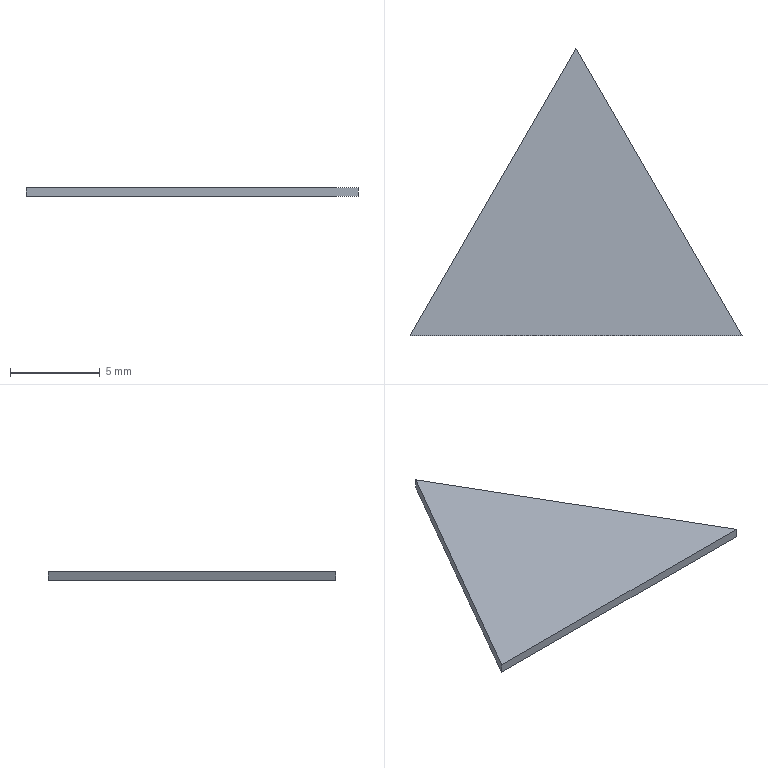Part | STEP file | [Hold-down mark] | 1 solid | 5 faces | box 18.475 x 16 x 0.5 mm | volume 73.901 mm3 | plane 5
STEP:
#1=CARTESIAN_POINT('',(0.,0.,0.5));
#2=VERTEX_POINT('',#1);
#3=CARTESIAN_POINT('',(9.238,16.,0.5));
#4=VERTEX_POINT('',#3);
#5=CARTESIAN_POINT('',(0.,0.,0.5));
#6=DIRECTION('',(0.5,0.866,0.));
#7=VECTOR('',#6,1000.);
#8=LINE('',#5,#7);
#9=EDGE_CURVE('',#2,#4,#8,.T.);
#10=ORIENTED_EDGE('',*,*,#9,.T.);
#11=CARTESIAN_POINT('',(9.238,16.,0.));
#12=VERTEX_POINT('',#11);
#13=CARTESIAN_POINT('',(9.238,16.,0.));
#14=DIRECTION('',(0.,0.,1.));
#15=VECTOR('',#14,1000.);
#16=LINE('',#13,#15);
#17=EDGE_CURVE('',#12,#4,#16,.T.);
#18=ORIENTED_EDGE('',*,*,#17,.F.);
#19=CARTESIAN_POINT('',(0.,0.,0.));
#20=VERTEX_POINT('',#19);
#21=CARTESIAN_POINT('',(0.,0.,0.));
#22=DIRECTION('',(0.5,0.866,0.));
#23=VECTOR('',#22,1000.);
#24=LINE('',#21,#23);
#25=EDGE_CURVE('',#20,#12,#24,.T.);
#26=ORIENTED_EDGE('',*,*,#25,.F.);
#27=CARTESIAN_POINT('',(0.,0.,0.));
#28=DIRECTION('',(0.,0.,1.));
#29=VECTOR('',#28,1000.);
#30=LINE('',#27,#29);
#31=EDGE_CURVE('',#20,#2,#30,.T.);
#32=ORIENTED_EDGE('',*,*,#31,.T.);
#33=EDGE_LOOP('',(#10,#18,#26,#32));
#34=FACE_OUTER_BOUND('',#33,.T.);
#35=CARTESIAN_POINT('',(0.,0.,0.));
#36=DIRECTION('',(0.866,-0.5,0.));
#37=DIRECTION('',(-0.5,-0.866,0.));
#38=AXIS2_PLACEMENT_3D('',#35,#36,#37);
#39=PLANE('',#38);
#40=ADVANCED_FACE('',(#34),#39,.F.);
#41=CARTESIAN_POINT('',(18.475,0.,0.5));
#42=VERTEX_POINT('',#41);
#43=CARTESIAN_POINT('',(9.238,16.,0.5));
#44=DIRECTION('',(0.5,-0.866,0.));
#45=VECTOR('',#44,1000.);
#46=LINE('',#43,#45);
#47=EDGE_CURVE('',#4,#42,#46,.T.);
#48=ORIENTED_EDGE('',*,*,#47,.T.);
#49=CARTESIAN_POINT('',(18.475,0.,0.));
#50=VERTEX_POINT('',#49);
#51=CARTESIAN_POINT('',(18.475,0.,0.));
#52=DIRECTION('',(0.,0.,1.));
#53=VECTOR('',#52,1000.);
#54=LINE('',#51,#53);
#55=EDGE_CURVE('',#50,#42,#54,.T.);
#56=ORIENTED_EDGE('',*,*,#55,.F.);
#57=CARTESIAN_POINT('',(9.238,16.,0.));
#58=DIRECTION('',(0.5,-0.866,0.));
#59=VECTOR('',#58,1000.);
#60=LINE('',#57,#59);
#61=EDGE_CURVE('',#12,#50,#60,.T.);
#62=ORIENTED_EDGE('',*,*,#61,.F.);
#63=ORIENTED_EDGE('',*,*,#17,.T.);
#64=EDGE_LOOP('',(#48,#56,#62,#63));
#65=FACE_OUTER_BOUND('',#64,.T.);
#66=CARTESIAN_POINT('',(9.238,16.,0.));
#67=DIRECTION('',(-0.866,-0.5,0.));
#68=DIRECTION('',(0.,0.,1.));
#69=AXIS2_PLACEMENT_3D('',#66,#67,#68);
#70=PLANE('',#69);
#71=ADVANCED_FACE('',(#65),#70,.F.);
#72=CARTESIAN_POINT('',(18.475,0.,0.5));
#73=DIRECTION('',(-1.,0.,0.));
#74=VECTOR('',#73,1000.);
#75=LINE('',#72,#74);
#76=EDGE_CURVE('',#42,#2,#75,.T.);
#77=ORIENTED_EDGE('',*,*,#76,.T.);
#78=ORIENTED_EDGE('',*,*,#31,.F.);
#79=CARTESIAN_POINT('',(18.475,0.,0.));
#80=DIRECTION('',(-1.,0.,0.));
#81=VECTOR('',#80,1000.);
#82=LINE('',#79,#81);
#83=EDGE_CURVE('',#50,#20,#82,.T.);
#84=ORIENTED_EDGE('',*,*,#83,.F.);
#85=ORIENTED_EDGE('',*,*,#55,.T.);
#86=EDGE_LOOP('',(#77,#78,#84,#85));
#87=FACE_OUTER_BOUND('',#86,.T.);
#88=CARTESIAN_POINT('',(18.475,0.,0.));
#89=DIRECTION('',(0.,1.,0.));
#90=DIRECTION('',(1.,0.,0.));
#91=AXIS2_PLACEMENT_3D('',#88,#89,#90);
#92=PLANE('',#91);
#93=ADVANCED_FACE('',(#87),#92,.F.);
#94=ORIENTED_EDGE('',*,*,#25,.T.);
#95=ORIENTED_EDGE('',*,*,#61,.T.);
#96=ORIENTED_EDGE('',*,*,#83,.T.);
#97=EDGE_LOOP('',(#94,#95,#96));
#98=FACE_OUTER_BOUND('',#97,.T.);
#99=CARTESIAN_POINT('',(128.356,-190.32,0.));
#100=DIRECTION('',(0.,0.,-1.));
#101=DIRECTION('',(-0.5,0.866,0.));
#102=AXIS2_PLACEMENT_3D('',#99,#100,#101);
#103=PLANE('',#102);
#104=ADVANCED_FACE('',(#98),#103,.T.);
#105=ORIENTED_EDGE('',*,*,#9,.F.);
#106=ORIENTED_EDGE('',*,*,#76,.F.);
#107=ORIENTED_EDGE('',*,*,#47,.F.);
#108=EDGE_LOOP('',(#105,#106,#107));
#109=FACE_OUTER_BOUND('',#108,.T.);
#110=CARTESIAN_POINT('',(128.356,-190.32,0.5));
#111=DIRECTION('',(0.,0.,-1.));
#112=DIRECTION('',(-0.5,0.866,0.));
#113=AXIS2_PLACEMENT_3D('',#110,#111,#112);
#114=PLANE('',#113);
#115=ADVANCED_FACE('',(#109),#114,.F.);
#116=CLOSED_SHELL('',(#40,#71,#93,#104,#115));
#117=MANIFOLD_SOLID_BREP('',#116);
#118=CARTESIAN_POINT('',(0.,0.,0.));
#119=DIRECTION('',(0.,0.,1.));
#120=DIRECTION('',(1.,0.,0.));
#121=AXIS2_PLACEMENT_3D('',#118,#119,#120);
#122=(LENGTH_UNIT()NAMED_UNIT(*)SI_UNIT(.MILLI.,.METRE.));
#123=UNCERTAINTY_MEASURE_WITH_UNIT(LENGTH_MEASURE(0.00001),#122,'','');
#124=(NAMED_UNIT(*)PLANE_ANGLE_UNIT()SI_UNIT($,.RADIAN.));
#125=(NAMED_UNIT(*)SI_UNIT($,.STERADIAN.)SOLID_ANGLE_UNIT());
#126=(GEOMETRIC_REPRESENTATION_CONTEXT(3)GLOBAL_UNCERTAINTY_ASSIGNED_CONTEXT((#123))GLOBAL_UNIT_ASSIGNED_CONTEXT((#122,#124,#125))REPRESENTATION_CONTEXT('',''));
#127=ADVANCED_BREP_SHAPE_REPRESENTATION('',(#117,#121),#126);